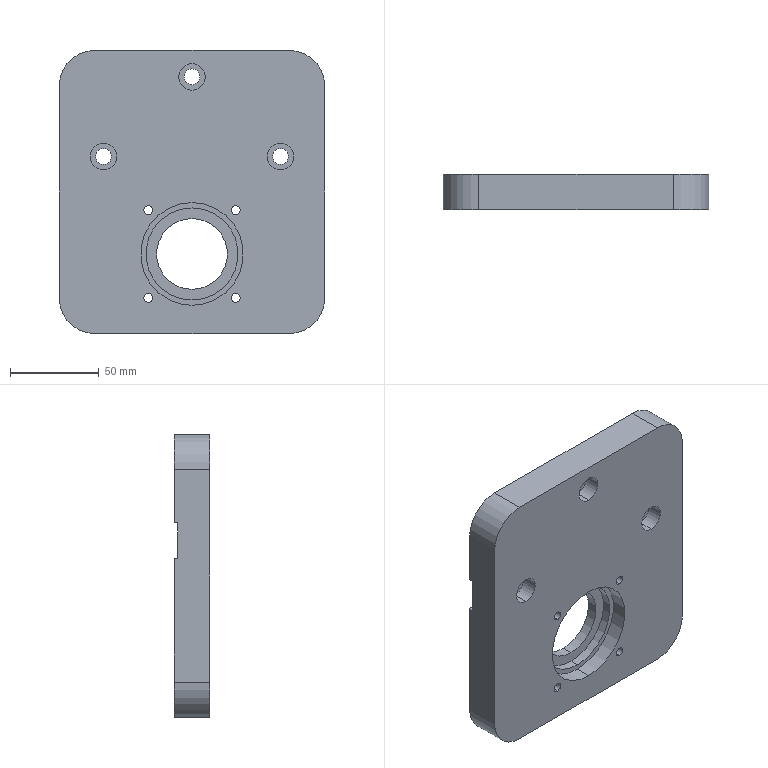Part | SolidWorks | features ICE 4, HoleWzd 2, Extrusion 1, Fillet 1 | 1 solid | 45 faces | box 150 x 20 x 160 mm | volume 417009 mm3 | cylinder 30 | plane 15 | commonest cylinder face diameters 5 x8 9 x6 15 x6 40 x6 52 x2 58 x2
STEP:
#1=CARTESIAN_POINT('',(125.,-11.,-52.5));
#2=VERTEX_POINT('',#1);
#3=CARTESIAN_POINT('',(125.,-11.,-67.5));
#4=VERTEX_POINT('',#3);
#5=CARTESIAN_POINT('',(125.,-11.,-60.));
#6=DIRECTION('',(0.,-1.,0.));
#7=DIRECTION('',(0.,0.,-1.));
#8=AXIS2_PLACEMENT_3D('',#5,#6,#7);
#9=CIRCLE('',#8,7.5);
#10=EDGE_CURVE('',#2,#4,#9,.T.);
#11=ORIENTED_EDGE('',*,*,#10,.F.);
#12=CARTESIAN_POINT('',(125.,-20.,-52.5));
#13=VERTEX_POINT('',#12);
#14=CARTESIAN_POINT('',(125.,-20.,-52.5));
#15=DIRECTION('',(0.,-1.,0.));
#16=VECTOR('',#15,1000.);
#17=LINE('',#14,#16);
#18=EDGE_CURVE('',#2,#13,#17,.T.);
#19=ORIENTED_EDGE('',*,*,#18,.T.);
#20=CARTESIAN_POINT('',(125.,-20.,-67.5));
#21=VERTEX_POINT('',#20);
#22=CARTESIAN_POINT('',(125.,-20.,-60.));
#23=DIRECTION('',(0.,-1.,0.));
#24=DIRECTION('',(0.,0.,-1.));
#25=AXIS2_PLACEMENT_3D('',#22,#23,#24);
#26=CIRCLE('',#25,7.5);
#27=EDGE_CURVE('',#13,#21,#26,.T.);
#28=ORIENTED_EDGE('',*,*,#27,.T.);
#29=CARTESIAN_POINT('',(125.,-20.,-67.5));
#30=DIRECTION('',(0.,-1.,0.));
#31=VECTOR('',#30,1000.);
#32=LINE('',#29,#31);
#33=EDGE_CURVE('',#4,#21,#32,.T.);
#34=ORIENTED_EDGE('',*,*,#33,.F.);
#35=EDGE_LOOP('',(#11,#19,#28,#34));
#36=FACE_OUTER_BOUND('',#35,.T.);
#37=CARTESIAN_POINT('',(125.,-20.,-60.));
#38=DIRECTION('',(0.,-1.,0.));
#39=DIRECTION('',(0.,0.,-1.));
#40=AXIS2_PLACEMENT_3D('',#37,#38,#39);
#41=CYLINDRICAL_SURFACE('',#40,7.5);
#42=ADVANCED_FACE('',(#36),#41,.F.);
#43=CARTESIAN_POINT('',(125.,-2.,-64.5));
#44=VERTEX_POINT('',#43);
#45=CARTESIAN_POINT('',(125.,-2.,-55.5));
#46=VERTEX_POINT('',#45);
#47=CARTESIAN_POINT('',(125.,-2.,-60.));
#48=DIRECTION('',(0.,1.,0.));
#49=DIRECTION('',(0.,0.,1.));
#50=AXIS2_PLACEMENT_3D('',#47,#48,#49);
#51=CIRCLE('',#50,4.5);
#52=EDGE_CURVE('',#44,#46,#51,.T.);
#53=ORIENTED_EDGE('',*,*,#52,.T.);
#54=CARTESIAN_POINT('',(125.,-11.,-55.5));
#55=VERTEX_POINT('',#54);
#56=CARTESIAN_POINT('',(125.,-20.,-55.5));
#57=DIRECTION('',(0.,-1.,0.));
#58=VECTOR('',#57,1000.);
#59=LINE('',#56,#58);
#60=EDGE_CURVE('',#46,#55,#59,.T.);
#61=ORIENTED_EDGE('',*,*,#60,.T.);
#62=CARTESIAN_POINT('',(125.,-11.,-64.5));
#63=VERTEX_POINT('',#62);
#64=CARTESIAN_POINT('',(125.,-11.,-60.));
#65=DIRECTION('',(0.,-1.,0.));
#66=DIRECTION('',(0.,0.,-1.));
#67=AXIS2_PLACEMENT_3D('',#64,#65,#66);
#68=CIRCLE('',#67,4.5);
#69=EDGE_CURVE('',#55,#63,#68,.T.);
#70=ORIENTED_EDGE('',*,*,#69,.T.);
#71=CARTESIAN_POINT('',(125.,-20.,-64.5));
#72=DIRECTION('',(0.,-1.,0.));
#73=VECTOR('',#72,1000.);
#74=LINE('',#71,#73);
#75=EDGE_CURVE('',#44,#63,#74,.T.);
#76=ORIENTED_EDGE('',*,*,#75,.F.);
#77=EDGE_LOOP('',(#53,#61,#70,#76));
#78=FACE_OUTER_BOUND('',#77,.T.);
#79=CARTESIAN_POINT('',(125.,-20.,-60.));
#80=DIRECTION('',(0.,-1.,0.));
#81=DIRECTION('',(0.,0.,-1.));
#82=AXIS2_PLACEMENT_3D('',#79,#80,#81);
#83=CYLINDRICAL_SURFACE('',#82,4.5);
#84=ADVANCED_FACE('',(#78),#83,.F.);
#85=CARTESIAN_POINT('',(25.,-11.,-52.5));
#86=VERTEX_POINT('',#85);
#87=CARTESIAN_POINT('',(25.,-11.,-67.5));
#88=VERTEX_POINT('',#87);
#89=CARTESIAN_POINT('',(25.,-11.,-60.));
#90=DIRECTION('',(0.,-1.,0.));
#91=DIRECTION('',(0.,0.,-1.));
#92=AXIS2_PLACEMENT_3D('',#89,#90,#91);
#93=CIRCLE('',#92,7.5);
#94=EDGE_CURVE('',#86,#88,#93,.T.);
#95=ORIENTED_EDGE('',*,*,#94,.F.);
#96=CARTESIAN_POINT('',(25.,-20.,-52.5));
#97=VERTEX_POINT('',#96);
#98=CARTESIAN_POINT('',(25.,-20.,-52.5));
#99=DIRECTION('',(0.,-1.,0.));
#100=VECTOR('',#99,1000.);
#101=LINE('',#98,#100);
#102=EDGE_CURVE('',#86,#97,#101,.T.);
#103=ORIENTED_EDGE('',*,*,#102,.T.);
#104=CARTESIAN_POINT('',(25.,-20.,-67.5));
#105=VERTEX_POINT('',#104);
#106=CARTESIAN_POINT('',(25.,-20.,-60.));
#107=DIRECTION('',(0.,-1.,0.));
#108=DIRECTION('',(0.,0.,-1.));
#109=AXIS2_PLACEMENT_3D('',#106,#107,#108);
#110=CIRCLE('',#109,7.5);
#111=EDGE_CURVE('',#97,#105,#110,.T.);
#112=ORIENTED_EDGE('',*,*,#111,.T.);
#113=CARTESIAN_POINT('',(25.,-20.,-67.5));
#114=DIRECTION('',(0.,-1.,0.));
#115=VECTOR('',#114,1000.);
#116=LINE('',#113,#115);
#117=EDGE_CURVE('',#88,#105,#116,.T.);
#118=ORIENTED_EDGE('',*,*,#117,.F.);
#119=EDGE_LOOP('',(#95,#103,#112,#118));
#120=FACE_OUTER_BOUND('',#119,.T.);
#121=CARTESIAN_POINT('',(25.,-20.,-60.));
#122=DIRECTION('',(0.,-1.,0.));
#123=DIRECTION('',(0.,0.,-1.));
#124=AXIS2_PLACEMENT_3D('',#121,#122,#123);
#125=CYLINDRICAL_SURFACE('',#124,7.5);
#126=ADVANCED_FACE('',(#120),#125,.F.);
#127=CARTESIAN_POINT('',(25.,-2.,-64.5));
#128=VERTEX_POINT('',#127);
#129=CARTESIAN_POINT('',(25.,-2.,-55.5));
#130=VERTEX_POINT('',#129);
#131=CARTESIAN_POINT('',(25.,-2.,-60.));
#132=DIRECTION('',(0.,1.,0.));
#133=DIRECTION('',(0.,0.,1.));
#134=AXIS2_PLACEMENT_3D('',#131,#132,#133);
#135=CIRCLE('',#134,4.5);
#136=EDGE_CURVE('',#128,#130,#135,.T.);
#137=ORIENTED_EDGE('',*,*,#136,.T.);
#138=CARTESIAN_POINT('',(25.,-11.,-55.5));
#139=VERTEX_POINT('',#138);
#140=CARTESIAN_POINT('',(25.,-20.,-55.5));
#141=DIRECTION('',(0.,-1.,0.));
#142=VECTOR('',#141,1000.);
#143=LINE('',#140,#142);
#144=EDGE_CURVE('',#130,#139,#143,.T.);
#145=ORIENTED_EDGE('',*,*,#144,.T.);
#146=CARTESIAN_POINT('',(25.,-11.,-64.5));
#147=VERTEX_POINT('',#146);
#148=CARTESIAN_POINT('',(25.,-11.,-60.));
#149=DIRECTION('',(0.,-1.,0.));
#150=DIRECTION('',(0.,0.,-1.));
#151=AXIS2_PLACEMENT_3D('',#148,#149,#150);
#152=CIRCLE('',#151,4.5);
#153=EDGE_CURVE('',#139,#147,#152,.T.);
#154=ORIENTED_EDGE('',*,*,#153,.T.);
#155=CARTESIAN_POINT('',(25.,-20.,-64.5));
#156=DIRECTION('',(0.,-1.,0.));
#157=VECTOR('',#156,1000.);
#158=LINE('',#155,#157);
#159=EDGE_CURVE('',#128,#147,#158,.T.);
#160=ORIENTED_EDGE('',*,*,#159,.F.);
#161=EDGE_LOOP('',(#137,#145,#154,#160));
#162=FACE_OUTER_BOUND('',#161,.T.);
#163=CARTESIAN_POINT('',(25.,-20.,-60.));
#164=DIRECTION('',(0.,-1.,0.));
#165=DIRECTION('',(0.,0.,-1.));
#166=AXIS2_PLACEMENT_3D('',#163,#164,#165);
#167=CYLINDRICAL_SURFACE('',#166,4.5);
#168=ADVANCED_FACE('',(#162),#167,.F.);
#169=CARTESIAN_POINT('',(75.,-11.,-7.5));
#170=VERTEX_POINT('',#169);
#171=CARTESIAN_POINT('',(75.,-11.,-22.5));
#172=VERTEX_POINT('',#171);
#173=CARTESIAN_POINT('',(75.,-11.,-15.));
#174=DIRECTION('',(0.,-1.,0.));
#175=DIRECTION('',(0.,0.,-1.));
#176=AXIS2_PLACEMENT_3D('',#173,#174,#175);
#177=CIRCLE('',#176,7.5);
#178=EDGE_CURVE('',#170,#172,#177,.T.);
#179=ORIENTED_EDGE('',*,*,#178,.F.);
#180=CARTESIAN_POINT('',(75.,-20.,-7.5));
#181=VERTEX_POINT('',#180);
#182=CARTESIAN_POINT('',(75.,-20.,-7.5));
#183=DIRECTION('',(0.,-1.,0.));
#184=VECTOR('',#183,1000.);
#185=LINE('',#182,#184);
#186=EDGE_CURVE('',#170,#181,#185,.T.);
#187=ORIENTED_EDGE('',*,*,#186,.T.);
#188=CARTESIAN_POINT('',(75.,-20.,-22.5));
#189=VERTEX_POINT('',#188);
#190=CARTESIAN_POINT('',(75.,-20.,-15.));
#191=DIRECTION('',(0.,-1.,0.));
#192=DIRECTION('',(0.,0.,-1.));
#193=AXIS2_PLACEMENT_3D('',#190,#191,#192);
#194=CIRCLE('',#193,7.5);
#195=EDGE_CURVE('',#181,#189,#194,.T.);
#196=ORIENTED_EDGE('',*,*,#195,.T.);
#197=CARTESIAN_POINT('',(75.,-20.,-22.5));
#198=DIRECTION('',(0.,-1.,0.));
#199=VECTOR('',#198,1000.);
#200=LINE('',#197,#199);
#201=EDGE_CURVE('',#172,#189,#200,.T.);
#202=ORIENTED_EDGE('',*,*,#201,.F.);
#203=EDGE_LOOP('',(#179,#187,#196,#202));
#204=FACE_OUTER_BOUND('',#203,.T.);
#205=CARTESIAN_POINT('',(75.,-20.,-15.));
#206=DIRECTION('',(0.,-1.,0.));
#207=DIRECTION('',(0.,0.,-1.));
#208=AXIS2_PLACEMENT_3D('',#205,#206,#207);
#209=CYLINDRICAL_SURFACE('',#208,7.5);
#210=ADVANCED_FACE('',(#204),#209,.F.);
#211=CARTESIAN_POINT('',(75.,0.,-10.5));
#212=VERTEX_POINT('',#211);
#213=CARTESIAN_POINT('',(75.,0.,-19.5));
#214=VERTEX_POINT('',#213);
#215=CARTESIAN_POINT('',(75.,0.,-15.));
#216=DIRECTION('',(0.,-1.,0.));
#217=DIRECTION('',(0.,0.,-1.));
#218=AXIS2_PLACEMENT_3D('',#215,#216,#217);
#219=CIRCLE('',#218,4.5);
#220=EDGE_CURVE('',#212,#214,#219,.T.);
#221=ORIENTED_EDGE('',*,*,#220,.F.);
#222=CARTESIAN_POINT('',(75.,-11.,-10.5));
#223=VERTEX_POINT('',#222);
#224=CARTESIAN_POINT('',(75.,-20.,-10.5));
#225=DIRECTION('',(0.,-1.,0.));
#226=VECTOR('',#225,1000.);
#227=LINE('',#224,#226);
#228=EDGE_CURVE('',#212,#223,#227,.T.);
#229=ORIENTED_EDGE('',*,*,#228,.T.);
#230=CARTESIAN_POINT('',(75.,-11.,-19.5));
#231=VERTEX_POINT('',#230);
#232=CARTESIAN_POINT('',(75.,-11.,-15.));
#233=DIRECTION('',(0.,-1.,0.));
#234=DIRECTION('',(0.,0.,-1.));
#235=AXIS2_PLACEMENT_3D('',#232,#233,#234);
#236=CIRCLE('',#235,4.5);
#237=EDGE_CURVE('',#223,#231,#236,.T.);
#238=ORIENTED_EDGE('',*,*,#237,.T.);
#239=CARTESIAN_POINT('',(75.,-20.,-19.5));
#240=DIRECTION('',(0.,-1.,0.));
#241=VECTOR('',#240,1000.);
#242=LINE('',#239,#241);
#243=EDGE_CURVE('',#214,#231,#242,.T.);
#244=ORIENTED_EDGE('',*,*,#243,.F.);
#245=EDGE_LOOP('',(#221,#229,#238,#244));
#246=FACE_OUTER_BOUND('',#245,.T.);
#247=CARTESIAN_POINT('',(75.,-20.,-15.));
#248=DIRECTION('',(0.,-1.,0.));
#249=DIRECTION('',(0.,0.,-1.));
#250=AXIS2_PLACEMENT_3D('',#247,#248,#249);
#251=CYLINDRICAL_SURFACE('',#250,4.5);
#252=ADVANCED_FACE('',(#246),#251,.F.);
#253=CARTESIAN_POINT('',(75.,-11.,-86.));
#254=VERTEX_POINT('',#253);
#255=CARTESIAN_POINT('',(75.,-11.,-144.));
#256=VERTEX_POINT('',#255);
#257=CARTESIAN_POINT('',(75.,-11.,-115.));
#258=DIRECTION('',(0.,-1.,0.));
#259=DIRECTION('',(0.,0.,-1.));
#260=AXIS2_PLACEMENT_3D('',#257,#258,#259);
#261=CIRCLE('',#260,29.);
#262=EDGE_CURVE('',#254,#256,#261,.T.);
#263=ORIENTED_EDGE('',*,*,#262,.F.);
#264=CARTESIAN_POINT('',(75.,-20.,-86.));
#265=VERTEX_POINT('',#264);
#266=CARTESIAN_POINT('',(75.,-11.,-86.));
#267=DIRECTION('',(0.,-1.,0.));
#268=VECTOR('',#267,1000.);
#269=LINE('',#266,#268);
#270=EDGE_CURVE('',#254,#265,#269,.T.);
#271=ORIENTED_EDGE('',*,*,#270,.T.);
#272=CARTESIAN_POINT('',(75.,-20.,-144.));
#273=VERTEX_POINT('',#272);
#274=CARTESIAN_POINT('',(75.,-20.,-115.));
#275=DIRECTION('',(0.,-1.,0.));
#276=DIRECTION('',(0.,0.,-1.));
#277=AXIS2_PLACEMENT_3D('',#274,#275,#276);
#278=CIRCLE('',#277,29.);
#279=EDGE_CURVE('',#265,#273,#278,.T.);
#280=ORIENTED_EDGE('',*,*,#279,.T.);
#281=CARTESIAN_POINT('',(75.,-11.,-144.));
#282=DIRECTION('',(0.,-1.,0.));
#283=VECTOR('',#282,1000.);
#284=LINE('',#281,#283);
#285=EDGE_CURVE('',#256,#273,#284,.T.);
#286=ORIENTED_EDGE('',*,*,#285,.F.);
#287=EDGE_LOOP('',(#263,#271,#280,#286));
#288=FACE_OUTER_BOUND('',#287,.T.);
#289=CARTESIAN_POINT('',(75.,-11.,-115.));
#290=DIRECTION('',(0.,-1.,0.));
#291=DIRECTION('',(0.,0.,-1.));
#292=AXIS2_PLACEMENT_3D('',#289,#290,#291);
#293=CYLINDRICAL_SURFACE('',#292,29.);
#294=ADVANCED_FACE('',(#288),#293,.F.);
#295=CARTESIAN_POINT('',(99.749,0.,-137.249));
#296=VERTEX_POINT('',#295);
#297=CARTESIAN_POINT('',(99.749,0.,-142.249));
#298=VERTEX_POINT('',#297);
#299=CARTESIAN_POINT('',(99.749,0.,-139.749));
#300=DIRECTION('',(0.,-1.,0.));
#301=DIRECTION('',(0.,0.,-1.));
#302=AXIS2_PLACEMENT_3D('',#299,#300,#301);
#303=CIRCLE('',#302,2.5);
#304=EDGE_CURVE('',#296,#298,#303,.T.);
#305=ORIENTED_EDGE('',*,*,#304,.F.);
#306=CARTESIAN_POINT('',(99.749,-20.,-137.249));
#307=VERTEX_POINT('',#306);
#308=CARTESIAN_POINT('',(99.749,-20.,-137.249));
#309=DIRECTION('',(0.,-1.,0.));
#310=VECTOR('',#309,1000.);
#311=LINE('',#308,#310);
#312=EDGE_CURVE('',#296,#307,#311,.T.);
#313=ORIENTED_EDGE('',*,*,#312,.T.);
#314=CARTESIAN_POINT('',(99.749,-20.,-142.249));
#315=VERTEX_POINT('',#314);
#316=CARTESIAN_POINT('',(99.749,-20.,-139.749));
#317=DIRECTION('',(0.,-1.,0.));
#318=DIRECTION('',(0.,0.,-1.));
#319=AXIS2_PLACEMENT_3D('',#316,#317,#318);
#320=CIRCLE('',#319,2.5);
#321=EDGE_CURVE('',#307,#315,#320,.T.);
#322=ORIENTED_EDGE('',*,*,#321,.T.);
#323=CARTESIAN_POINT('',(99.749,-20.,-142.249));
#324=DIRECTION('',(0.,-1.,0.));
#325=VECTOR('',#324,1000.);
#326=LINE('',#323,#325);
#327=EDGE_CURVE('',#298,#315,#326,.T.);
#328=ORIENTED_EDGE('',*,*,#327,.F.);
#329=EDGE_LOOP('',(#305,#313,#322,#328));
#330=FACE_OUTER_BOUND('',#329,.T.);
#331=CARTESIAN_POINT('',(99.749,-20.,-139.749));
#332=DIRECTION('',(0.,-1.,0.));
#333=DIRECTION('',(0.,0.,-1.));
#334=AXIS2_PLACEMENT_3D('',#331,#332,#333);
#335=CYLINDRICAL_SURFACE('',#334,2.5);
#336=ADVANCED_FACE('',(#330),#335,.F.);
#337=CARTESIAN_POINT('',(50.251,0.,-137.249));
#338=VERTEX_POINT('',#337);
#339=CARTESIAN_POINT('',(50.251,0.,-142.249));
#340=VERTEX_POINT('',#339);
#341=CARTESIAN_POINT('',(50.251,0.,-139.749));
#342=DIRECTION('',(0.,-1.,0.));
#343=DIRECTION('',(0.,0.,-1.));
#344=AXIS2_PLACEMENT_3D('',#341,#342,#343);
#345=CIRCLE('',#344,2.5);
#346=EDGE_CURVE('',#338,#340,#345,.T.);
#347=ORIENTED_EDGE('',*,*,#346,.F.);
#348=CARTESIAN_POINT('',(50.251,-20.,-137.249));
#349=VERTEX_POINT('',#348);
#350=CARTESIAN_POINT('',(50.251,-20.,-137.249));
#351=DIRECTION('',(0.,-1.,0.));
#352=VECTOR('',#351,1000.);
#353=LINE('',#350,#352);
#354=EDGE_CURVE('',#338,#349,#353,.T.);
#355=ORIENTED_EDGE('',*,*,#354,.T.);
#356=CARTESIAN_POINT('',(50.251,-20.,-142.249));
#357=VERTEX_POINT('',#356);
#358=CARTESIAN_POINT('',(50.251,-20.,-139.749));
#359=DIRECTION('',(0.,-1.,0.));
#360=DIRECTION('',(0.,0.,-1.));
#361=AXIS2_PLACEMENT_3D('',#358,#359,#360);
#362=CIRCLE('',#361,2.5);
#363=EDGE_CURVE('',#349,#357,#362,.T.);
#364=ORIENTED_EDGE('',*,*,#363,.T.);
#365=CARTESIAN_POINT('',(50.251,-20.,-142.249));
#366=DIRECTION('',(0.,-1.,0.));
#367=VECTOR('',#366,1000.);
#368=LINE('',#365,#367);
#369=EDGE_CURVE('',#340,#357,#368,.T.);
#370=ORIENTED_EDGE('',*,*,#369,.F.);
#371=EDGE_LOOP('',(#347,#355,#364,#370));
#372=FACE_OUTER_BOUND('',#371,.T.);
#373=CARTESIAN_POINT('',(50.251,-20.,-139.749));
#374=DIRECTION('',(0.,-1.,0.));
#375=DIRECTION('',(0.,0.,-1.));
#376=AXIS2_PLACEMENT_3D('',#373,#374,#375);
#377=CYLINDRICAL_SURFACE('',#376,2.5);
#378=ADVANCED_FACE('',(#372),#377,.F.);
#379=CARTESIAN_POINT('',(50.251,0.,-87.751));
#380=VERTEX_POINT('',#379);
#381=CARTESIAN_POINT('',(50.251,0.,-92.751));
#382=VERTEX_POINT('',#381);
#383=CARTESIAN_POINT('',(50.251,0.,-90.251));
#384=DIRECTION('',(0.,-1.,0.));
#385=DIRECTION('',(0.,0.,-1.));
#386=AXIS2_PLACEMENT_3D('',#383,#384,#385);
#387=CIRCLE('',#386,2.5);
#388=EDGE_CURVE('',#380,#382,#387,.T.);
#389=ORIENTED_EDGE('',*,*,#388,.F.);
#390=CARTESIAN_POINT('',(50.251,-20.,-87.751));
#391=VERTEX_POINT('',#390);
#392=CARTESIAN_POINT('',(50.251,-20.,-87.751));
#393=DIRECTION('',(0.,-1.,0.));
#394=VECTOR('',#393,1000.);
#395=LINE('',#392,#394);
#396=EDGE_CURVE('',#380,#391,#395,.T.);
#397=ORIENTED_EDGE('',*,*,#396,.T.);
#398=CARTESIAN_POINT('',(50.251,-20.,-92.751));
#399=VERTEX_POINT('',#398);
#400=CARTESIAN_POINT('',(50.251,-20.,-90.251));
#401=DIRECTION('',(0.,-1.,0.));
#402=DIRECTION('',(0.,0.,-1.));
#403=AXIS2_PLACEMENT_3D('',#400,#401,#402);
#404=CIRCLE('',#403,2.5);
#405=EDGE_CURVE('',#391,#399,#404,.T.);
#406=ORIENTED_EDGE('',*,*,#405,.T.);
#407=CARTESIAN_POINT('',(50.251,-20.,-92.751));
#408=DIRECTION('',(0.,-1.,0.));
#409=VECTOR('',#408,1000.);
#410=LINE('',#407,#409);
#411=EDGE_CURVE('',#382,#399,#410,.T.);
#412=ORIENTED_EDGE('',*,*,#411,.F.);
#413=EDGE_LOOP('',(#389,#397,#406,#412));
#414=FACE_OUTER_BOUND('',#413,.T.);
#415=CARTESIAN_POINT('',(50.251,-20.,-90.251));
#416=DIRECTION('',(0.,-1.,0.));
#417=DIRECTION('',(0.,0.,-1.));
#418=AXIS2_PLACEMENT_3D('',#415,#416,#417);
#419=CYLINDRICAL_SURFACE('',#418,2.5);
#420=ADVANCED_FACE('',(#414),#419,.F.);
#421=CARTESIAN_POINT('',(99.749,0.,-87.751));
#422=VERTEX_POINT('',#421);
#423=CARTESIAN_POINT('',(99.749,0.,-92.751));
#424=VERTEX_POINT('',#423);
#425=CARTESIAN_POINT('',(99.749,0.,-90.251));
#426=DIRECTION('',(0.,-1.,0.));
#427=DIRECTION('',(0.,0.,-1.));
#428=AXIS2_PLACEMENT_3D('',#425,#426,#427);
#429=CIRCLE('',#428,2.5);
#430=EDGE_CURVE('',#422,#424,#429,.T.);
#431=ORIENTED_EDGE('',*,*,#430,.F.);
#432=CARTESIAN_POINT('',(99.749,-20.,-87.751));
#433=VERTEX_POINT('',#432);
#434=CARTESIAN_POINT('',(99.749,-20.,-87.751));
#435=DIRECTION('',(0.,-1.,0.));
#436=VECTOR('',#435,1000.);
#437=LINE('',#434,#436);
#438=EDGE_CURVE('',#422,#433,#437,.T.);
#439=ORIENTED_EDGE('',*,*,#438,.T.);
#440=CARTESIAN_POINT('',(99.749,-20.,-92.751));
#441=VERTEX_POINT('',#440);
#442=CARTESIAN_POINT('',(99.749,-20.,-90.251));
#443=DIRECTION('',(0.,-1.,0.));
#444=DIRECTION('',(0.,0.,-1.));
#445=AXIS2_PLACEMENT_3D('',#442,#443,#444);
#446=CIRCLE('',#445,2.5);
#447=EDGE_CURVE('',#433,#441,#446,.T.);
#448=ORIENTED_EDGE('',*,*,#447,.T.);
#449=CARTESIAN_POINT('',(99.749,-20.,-92.751));
#450=DIRECTION('',(0.,-1.,0.));
#451=VECTOR('',#450,1000.);
#452=LINE('',#449,#451);
#453=EDGE_CURVE('',#424,#441,#452,.T.);
#454=ORIENTED_EDGE('',*,*,#453,.F.);
#455=EDGE_LOOP('',(#431,#439,#448,#454));
#456=FACE_OUTER_BOUND('',#455,.T.);
#457=CARTESIAN_POINT('',(99.749,-20.,-90.251));
#458=DIRECTION('',(0.,-1.,0.));
#459=DIRECTION('',(0.,0.,-1.));
#460=AXIS2_PLACEMENT_3D('',#457,#458,#459);
#461=CYLINDRICAL_SURFACE('',#460,2.5);
#462=ADVANCED_FACE('',(#456),#461,.F.);
#463=CARTESIAN_POINT('',(75.,0.,-95.));
#464=VERTEX_POINT('',#463);
#465=CARTESIAN_POINT('',(75.,0.,-135.));
#466=VERTEX_POINT('',#465);
#467=CARTESIAN_POINT('',(75.,0.,-115.));
#468=DIRECTION('',(0.,-1.,0.));
#469=DIRECTION('',(0.,0.,-1.));
#470=AXIS2_PLACEMENT_3D('',#467,#468,#469);
#471=CIRCLE('',#470,20.);
#472=EDGE_CURVE('',#464,#466,#471,.T.);
#473=ORIENTED_EDGE('',*,*,#472,.F.);
#474=CARTESIAN_POINT('',(75.,-6.,-95.));
#475=VERTEX_POINT('',#474);
#476=CARTESIAN_POINT('',(75.,8.,-95.));
#477=DIRECTION('',(0.,-1.,0.));
#478=VECTOR('',#477,1000.);
#479=LINE('',#476,#478);
#480=EDGE_CURVE('',#464,#475,#479,.T.);
#481=ORIENTED_EDGE('',*,*,#480,.T.);
#482=CARTESIAN_POINT('',(75.,-6.,-135.));
#483=VERTEX_POINT('',#482);
#484=CARTESIAN_POINT('',(75.,-6.,-115.));
#485=DIRECTION('',(0.,-1.,0.));
#486=DIRECTION('',(0.,0.,-1.));
#487=AXIS2_PLACEMENT_3D('',#484,#485,#486);
#488=CIRCLE('',#487,20.);
#489=EDGE_CURVE('',#475,#483,#488,.T.);
#490=ORIENTED_EDGE('',*,*,#489,.T.);
#491=CARTESIAN_POINT('',(75.,8.,-135.));
#492=DIRECTION('',(0.,-1.,0.));
#493=VECTOR('',#492,1000.);
#494=LINE('',#491,#493);
#495=EDGE_CURVE('',#466,#483,#494,.T.);
#496=ORIENTED_EDGE('',*,*,#495,.F.);
#497=EDGE_LOOP('',(#473,#481,#490,#496));
#498=FACE_OUTER_BOUND('',#497,.T.);
#499=CARTESIAN_POINT('',(75.,8.,-115.));
#500=DIRECTION('',(0.,-1.,0.));
#501=DIRECTION('',(0.,0.,-1.));
#502=AXIS2_PLACEMENT_3D('',#499,#500,#501);
#503=CYLINDRICAL_SURFACE('',#502,20.);
#504=ADVANCED_FACE('',(#498),#503,.F.);
#505=CARTESIAN_POINT('',(75.,-6.,-89.));
#506=VERTEX_POINT('',#505);
#507=CARTESIAN_POINT('',(75.,-6.,-141.));
#508=VERTEX_POINT('',#507);
#509=CARTESIAN_POINT('',(75.,-6.,-115.));
#510=DIRECTION('',(0.,-1.,0.));
#511=DIRECTION('',(0.,0.,-1.));
#512=AXIS2_PLACEMENT_3D('',#509,#510,#511);
#513=CIRCLE('',#512,26.);
#514=EDGE_CURVE('',#506,#508,#513,.T.);
#515=ORIENTED_EDGE('',*,*,#514,.F.);
#516=CARTESIAN_POINT('',(75.,-11.,-89.));
#517=VERTEX_POINT('',#516);
#518=CARTESIAN_POINT('',(75.,-6.,-89.));
#519=DIRECTION('',(0.,-1.,0.));
#520=VECTOR('',#519,1000.);
#521=LINE('',#518,#520);
#522=EDGE_CURVE('',#506,#517,#521,.T.);
#523=ORIENTED_EDGE('',*,*,#522,.T.);
#524=CARTESIAN_POINT('',(75.,-11.,-141.));
#525=VERTEX_POINT('',#524);
#526=CARTESIAN_POINT('',(75.,-11.,-115.));
#527=DIRECTION('',(0.,1.,0.));
#528=DIRECTION('',(0.,0.,-1.));
#529=AXIS2_PLACEMENT_3D('',#526,#527,#528);
#530=CIRCLE('',#529,26.);
#531=EDGE_CURVE('',#525,#517,#530,.T.);
#532=ORIENTED_EDGE('',*,*,#531,.F.);
#533=CARTESIAN_POINT('',(75.,-6.,-141.));
#534=DIRECTION('',(0.,-1.,0.));
#535=VECTOR('',#534,1000.);
#536=LINE('',#533,#535);
#537=EDGE_CURVE('',#508,#525,#536,.T.);
#538=ORIENTED_EDGE('',*,*,#537,.F.);
#539=EDGE_LOOP('',(#515,#523,#532,#538));
#540=FACE_OUTER_BOUND('',#539,.T.);
#541=CARTESIAN_POINT('',(75.,-6.,-115.));
#542=DIRECTION('',(0.,-1.,0.));
#543=DIRECTION('',(0.,0.,-1.));
#544=AXIS2_PLACEMENT_3D('',#541,#542,#543);
#545=CYLINDRICAL_SURFACE('',#544,26.);
#546=ADVANCED_FACE('',(#540),#545,.F.);
#547=CARTESIAN_POINT('',(75.,0.,-115.));
#548=DIRECTION('',(0.,-1.,0.));
#549=DIRECTION('',(0.,0.,-1.));
#550=AXIS2_PLACEMENT_3D('',#547,#548,#549);
#551=CIRCLE('',#550,20.);
#552=EDGE_CURVE('',#466,#464,#551,.T.);
#553=ORIENTED_EDGE('',*,*,#552,.T.);
#554=ORIENTED_EDGE('',*,*,#472,.T.);
#555=EDGE_LOOP('',(#553,#554));
#556=FACE_BOUND('',#555,.T.);
#557=CARTESIAN_POINT('',(99.749,0.,-90.251));
#558=DIRECTION('',(0.,-1.,0.));
#559=DIRECTION('',(0.,0.,-1.));
#560=AXIS2_PLACEMENT_3D('',#557,#558,#559);
#561=CIRCLE('',#560,2.5);
#562=EDGE_CURVE('',#424,#422,#561,.T.);
#563=ORIENTED_EDGE('',*,*,#562,.T.);
#564=ORIENTED_EDGE('',*,*,#430,.T.);
#565=EDGE_LOOP('',(#563,#564));
#566=FACE_BOUND('',#565,.T.);
#567=CARTESIAN_POINT('',(50.251,0.,-90.251));
#568=DIRECTION('',(0.,-1.,0.));
#569=DIRECTION('',(0.,0.,-1.));
#570=AXIS2_PLACEMENT_3D('',#567,#568,#569);
#571=CIRCLE('',#570,2.5);
#572=EDGE_CURVE('',#382,#380,#571,.T.);
#573=ORIENTED_EDGE('',*,*,#572,.T.);
#574=ORIENTED_EDGE('',*,*,#388,.T.);
#575=EDGE_LOOP('',(#573,#574));
#576=FACE_BOUND('',#575,.T.);
#577=CARTESIAN_POINT('',(50.251,0.,-139.749));
#578=DIRECTION('',(0.,-1.,0.));
#579=DIRECTION('',(0.,0.,-1.));
#580=AXIS2_PLACEMENT_3D('',#577,#578,#579);
#581=CIRCLE('',#580,2.5);
#582=EDGE_CURVE('',#340,#338,#581,.T.);
#583=ORIENTED_EDGE('',*,*,#582,.T.);
#584=ORIENTED_EDGE('',*,*,#346,.T.);
#585=EDGE_LOOP('',(#583,#584));
#586=FACE_BOUND('',#585,.T.);
#587=CARTESIAN_POINT('',(99.749,0.,-139.749));
#588=DIRECTION('',(0.,-1.,0.));
#589=DIRECTION('',(0.,0.,-1.));
#590=AXIS2_PLACEMENT_3D('',#587,#588,#589);
#591=CIRCLE('',#590,2.5);
#592=EDGE_CURVE('',#298,#296,#591,.T.);
#593=ORIENTED_EDGE('',*,*,#592,.T.);
#594=ORIENTED_EDGE('',*,*,#304,.T.);
#595=EDGE_LOOP('',(#593,#594));
#596=FACE_BOUND('',#595,.T.);
#597=CARTESIAN_POINT('',(0.,0.,-70.));
#598=VERTEX_POINT('',#597);
#599=CARTESIAN_POINT('',(0.,0.,-140.));
#600=VERTEX_POINT('',#599);
#601=CARTESIAN_POINT('',(0.,0.,0.));
#602=DIRECTION('',(0.,0.,-1.));
#603=VECTOR('',#602,1000.);
#604=LINE('',#601,#603);
#605=EDGE_CURVE('',#598,#600,#604,.T.);
#606=ORIENTED_EDGE('',*,*,#605,.F.);
#607=CARTESIAN_POINT('',(150.,0.,-70.));
#608=VERTEX_POINT('',#607);
#609=CARTESIAN_POINT('',(0.,0.,-70.));
#610=DIRECTION('',(-1.,0.,0.));
#611=VECTOR('',#610,1000.);
#612=LINE('',#609,#611);
#613=EDGE_CURVE('',#608,#598,#612,.T.);
#614=ORIENTED_EDGE('',*,*,#613,.F.);
#615=CARTESIAN_POINT('',(150.,0.,-140.));
#616=VERTEX_POINT('',#615);
#617=CARTESIAN_POINT('',(150.,0.,0.));
#618=DIRECTION('',(0.,0.,1.));
#619=VECTOR('',#618,1000.);
#620=LINE('',#617,#619);
#621=EDGE_CURVE('',#616,#608,#620,.T.);
#622=ORIENTED_EDGE('',*,*,#621,.F.);
#623=CARTESIAN_POINT('',(130.,0.,-160.));
#624=VERTEX_POINT('',#623);
#625=CARTESIAN_POINT('',(130.,0.,-140.));
#626=DIRECTION('',(0.,1.,0.));
#627=DIRECTION('',(0.,0.,-1.));
#628=AXIS2_PLACEMENT_3D('',#625,#626,#627);
#629=CIRCLE('',#628,20.);
#630=EDGE_CURVE('',#616,#624,#629,.T.);
#631=ORIENTED_EDGE('',*,*,#630,.T.);
#632=CARTESIAN_POINT('',(20.,0.,-160.));
#633=VERTEX_POINT('',#632);
#634=CARTESIAN_POINT('',(0.,0.,-160.));
#635=DIRECTION('',(1.,0.,0.));
#636=VECTOR('',#635,1000.);
#637=LINE('',#634,#636);
#638=EDGE_CURVE('',#633,#624,#637,.T.);
#639=ORIENTED_EDGE('',*,*,#638,.F.);
#640=CARTESIAN_POINT('',(20.,0.,-140.));
#641=DIRECTION('',(0.,1.,0.));
#642=DIRECTION('',(0.,0.,-1.));
#643=AXIS2_PLACEMENT_3D('',#640,#641,#642);
#644=CIRCLE('',#643,20.);
#645=EDGE_CURVE('',#633,#600,#644,.T.);
#646=ORIENTED_EDGE('',*,*,#645,.T.);
#647=EDGE_LOOP('',(#606,#614,#622,#631,#639,#646));
#648=FACE_OUTER_BOUND('',#647,.T.);
#649=CARTESIAN_POINT('',(0.,0.,0.));
#650=DIRECTION('',(0.,-1.,0.));
#651=DIRECTION('',(0.,0.,-1.));
#652=AXIS2_PLACEMENT_3D('',#649,#650,#651);
#653=PLANE('',#652);
#654=ADVANCED_FACE('',(#556,#566,#576,#586,#596,#648),#653,.F.);
#655=ORIENTED_EDGE('',*,*,#522,.F.);
#656=CARTESIAN_POINT('',(75.,-6.,-115.));
#657=DIRECTION('',(0.,-1.,0.));
#658=DIRECTION('',(0.,0.,-1.));
#659=AXIS2_PLACEMENT_3D('',#656,#657,#658);
#660=CIRCLE('',#659,26.);
#661=EDGE_CURVE('',#508,#506,#660,.T.);
#662=ORIENTED_EDGE('',*,*,#661,.F.);
#663=ORIENTED_EDGE('',*,*,#537,.T.);
#664=CARTESIAN_POINT('',(75.,-11.,-115.));
#665=DIRECTION('',(0.,1.,0.));
#666=DIRECTION('',(0.,0.,-1.));
#667=AXIS2_PLACEMENT_3D('',#664,#665,#666);
#668=CIRCLE('',#667,26.);
#669=EDGE_CURVE('',#517,#525,#668,.T.);
#670=ORIENTED_EDGE('',*,*,#669,.F.);
#671=EDGE_LOOP('',(#655,#662,#663,#670));
#672=FACE_OUTER_BOUND('',#671,.T.);
#673=CARTESIAN_POINT('',(75.,-6.,-115.));
#674=DIRECTION('',(0.,-1.,0.));
#675=DIRECTION('',(0.,0.,-1.));
#676=AXIS2_PLACEMENT_3D('',#673,#674,#675);
#677=CYLINDRICAL_SURFACE('',#676,26.);
#678=ADVANCED_FACE('',(#672),#677,.F.);
#679=CARTESIAN_POINT('',(0.,-2.,-70.));
#680=VERTEX_POINT('',#679);
#681=CARTESIAN_POINT('',(0.,-2.,-50.));
#682=VERTEX_POINT('',#681);
#683=CARTESIAN_POINT('',(0.,-2.,-70.));
#684=DIRECTION('',(0.,0.,1.));
#685=VECTOR('',#684,1000.);
#686=LINE('',#683,#685);
#687=EDGE_CURVE('',#680,#682,#686,.T.);
#688=ORIENTED_EDGE('',*,*,#687,.F.);
#689=CARTESIAN_POINT('',(0.,-2.,-70.));
#690=DIRECTION('',(0.,1.,0.));
#691=VECTOR('',#690,1000.);
#692=LINE('',#689,#691);
#693=EDGE_CURVE('',#680,#598,#692,.T.);
#694=ORIENTED_EDGE('',*,*,#693,.T.);
#695=ORIENTED_EDGE('',*,*,#605,.T.);
#696=CARTESIAN_POINT('',(0.,-20.,-140.));
#697=VERTEX_POINT('',#696);
#698=CARTESIAN_POINT('',(0.,-20.,-140.));
#699=DIRECTION('',(0.,-1.,0.));
#700=VECTOR('',#699,1000.);
#701=LINE('',#698,#700);
#702=EDGE_CURVE('',#600,#697,#701,.T.);
#703=ORIENTED_EDGE('',*,*,#702,.T.);
#704=CARTESIAN_POINT('',(0.,-20.,-20.));
#705=VERTEX_POINT('',#704);
#706=CARTESIAN_POINT('',(0.,-20.,0.));
#707=DIRECTION('',(0.,0.,-1.));
#708=VECTOR('',#707,1000.);
#709=LINE('',#706,#708);
#710=EDGE_CURVE('',#705,#697,#709,.T.);
#711=ORIENTED_EDGE('',*,*,#710,.F.);
#712=CARTESIAN_POINT('',(0.,0.,-20.));
#713=VERTEX_POINT('',#712);
#714=CARTESIAN_POINT('',(0.,-20.,-20.));
#715=DIRECTION('',(0.,1.,0.));
#716=VECTOR('',#715,1000.);
#717=LINE('',#714,#716);
#718=EDGE_CURVE('',#705,#713,#717,.T.);
#719=ORIENTED_EDGE('',*,*,#718,.T.);
#720=CARTESIAN_POINT('',(0.,0.,-50.));
#721=VERTEX_POINT('',#720);
#722=CARTESIAN_POINT('',(0.,0.,0.));
#723=DIRECTION('',(0.,0.,-1.));
#724=VECTOR('',#723,1000.);
#725=LINE('',#722,#724);
#726=EDGE_CURVE('',#713,#721,#725,.T.);
#727=ORIENTED_EDGE('',*,*,#726,.T.);
#728=CARTESIAN_POINT('',(0.,-2.,-50.));
#729=DIRECTION('',(0.,1.,0.));
#730=VECTOR('',#729,1000.);
#731=LINE('',#728,#730);
#732=EDGE_CURVE('',#682,#721,#731,.T.);
#733=ORIENTED_EDGE('',*,*,#732,.F.);
#734=EDGE_LOOP('',(#688,#694,#695,#703,#711,#719,#727,#733));
#735=FACE_OUTER_BOUND('',#734,.T.);
#736=CARTESIAN_POINT('',(0.,-20.,0.));
#737=DIRECTION('',(1.,0.,0.));
#738=DIRECTION('',(0.,0.,-1.));
#739=AXIS2_PLACEMENT_3D('',#736,#737,#738);
#740=PLANE('',#739);
#741=ADVANCED_FACE('',(#735),#740,.F.);
#742=ORIENTED_EDGE('',*,*,#638,.T.);
#743=CARTESIAN_POINT('',(130.,-20.,-160.));
#744=VERTEX_POINT('',#743);
#745=CARTESIAN_POINT('',(130.,-20.,-160.));
#746=DIRECTION('',(0.,-1.,0.));
#747=VECTOR('',#746,1000.);
#748=LINE('',#745,#747);
#749=EDGE_CURVE('',#624,#744,#748,.T.);
#750=ORIENTED_EDGE('',*,*,#749,.T.);
#751=CARTESIAN_POINT('',(20.,-20.,-160.));
#752=VERTEX_POINT('',#751);
#753=CARTESIAN_POINT('',(0.,-20.,-160.));
#754=DIRECTION('',(1.,0.,0.));
#755=VECTOR('',#754,1000.);
#756=LINE('',#753,#755);
#757=EDGE_CURVE('',#752,#744,#756,.T.);
#758=ORIENTED_EDGE('',*,*,#757,.F.);
#759=CARTESIAN_POINT('',(20.,-20.,-160.));
#760=DIRECTION('',(0.,1.,0.));
#761=VECTOR('',#760,1000.);
#762=LINE('',#759,#761);
#763=EDGE_CURVE('',#752,#633,#762,.T.);
#764=ORIENTED_EDGE('',*,*,#763,.T.);
#765=EDGE_LOOP('',(#742,#750,#758,#764));
#766=FACE_OUTER_BOUND('',#765,.T.);
#767=CARTESIAN_POINT('',(0.,-20.,-160.));
#768=DIRECTION('',(0.,0.,1.));
#769=DIRECTION('',(1.,0.,0.));
#770=AXIS2_PLACEMENT_3D('',#767,#768,#769);
#771=PLANE('',#770);
#772=ADVANCED_FACE('',(#766),#771,.F.);
#773=ORIENTED_EDGE('',*,*,#621,.T.);
#774=CARTESIAN_POINT('',(150.,-2.,-70.));
#775=VERTEX_POINT('',#774);
#776=CARTESIAN_POINT('',(150.,-2.,-70.));
#777=DIRECTION('',(0.,1.,0.));
#778=VECTOR('',#777,1000.);
#779=LINE('',#776,#778);
#780=EDGE_CURVE('',#775,#608,#779,.T.);
#781=ORIENTED_EDGE('',*,*,#780,.F.);
#782=CARTESIAN_POINT('',(150.,-2.,-50.));
#783=VERTEX_POINT('',#782);
#784=CARTESIAN_POINT('',(150.,-2.,-70.));
#785=DIRECTION('',(0.,0.,-1.));
#786=VECTOR('',#785,1000.);
#787=LINE('',#784,#786);
#788=EDGE_CURVE('',#783,#775,#787,.T.);
#789=ORIENTED_EDGE('',*,*,#788,.F.);
#790=CARTESIAN_POINT('',(150.,0.,-50.));
#791=VERTEX_POINT('',#790);
#792=CARTESIAN_POINT('',(150.,-2.,-50.));
#793=DIRECTION('',(0.,1.,0.));
#794=VECTOR('',#793,1000.);
#795=LINE('',#792,#794);
#796=EDGE_CURVE('',#783,#791,#795,.T.);
#797=ORIENTED_EDGE('',*,*,#796,.T.);
#798=CARTESIAN_POINT('',(150.,0.,-20.));
#799=VERTEX_POINT('',#798);
#800=CARTESIAN_POINT('',(150.,0.,0.));
#801=DIRECTION('',(0.,0.,1.));
#802=VECTOR('',#801,1000.);
#803=LINE('',#800,#802);
#804=EDGE_CURVE('',#791,#799,#803,.T.);
#805=ORIENTED_EDGE('',*,*,#804,.T.);
#806=CARTESIAN_POINT('',(150.,-20.,-20.));
#807=VERTEX_POINT('',#806);
#808=CARTESIAN_POINT('',(150.,-20.,-20.));
#809=DIRECTION('',(0.,-1.,0.));
#810=VECTOR('',#809,1000.);
#811=LINE('',#808,#810);
#812=EDGE_CURVE('',#799,#807,#811,.T.);
#813=ORIENTED_EDGE('',*,*,#812,.T.);
#814=CARTESIAN_POINT('',(150.,-20.,-140.));
#815=VERTEX_POINT('',#814);
#816=CARTESIAN_POINT('',(150.,-20.,0.));
#817=DIRECTION('',(0.,0.,1.));
#818=VECTOR('',#817,1000.);
#819=LINE('',#816,#818);
#820=EDGE_CURVE('',#815,#807,#819,.T.);
#821=ORIENTED_EDGE('',*,*,#820,.F.);
#822=CARTESIAN_POINT('',(150.,-20.,-140.));
#823=DIRECTION('',(0.,1.,0.));
#824=VECTOR('',#823,1000.);
#825=LINE('',#822,#824);
#826=EDGE_CURVE('',#815,#616,#825,.T.);
#827=ORIENTED_EDGE('',*,*,#826,.T.);
#828=EDGE_LOOP('',(#773,#781,#789,#797,#805,#813,#821,#827));
#829=FACE_OUTER_BOUND('',#828,.T.);
#830=CARTESIAN_POINT('',(150.,-20.,0.));
#831=DIRECTION('',(-1.,0.,0.));
#832=DIRECTION('',(0.,0.,1.));
#833=AXIS2_PLACEMENT_3D('',#830,#831,#832);
#834=PLANE('',#833);
#835=ADVANCED_FACE('',(#829),#834,.F.);
#836=CARTESIAN_POINT('',(130.,-20.,0.));
#837=VERTEX_POINT('',#836);
#838=CARTESIAN_POINT('',(20.,-20.,0.));
#839=VERTEX_POINT('',#838);
#840=CARTESIAN_POINT('',(0.,-20.,0.));
#841=DIRECTION('',(-1.,0.,0.));
#842=VECTOR('',#841,1000.);
#843=LINE('',#840,#842);
#844=EDGE_CURVE('',#837,#839,#843,.T.);
#845=ORIENTED_EDGE('',*,*,#844,.F.);
#846=CARTESIAN_POINT('',(130.,0.,0.));
#847=VERTEX_POINT('',#846);
#848=CARTESIAN_POINT('',(130.,-20.,0.));
#849=DIRECTION('',(0.,1.,0.));
#850=VECTOR('',#849,1000.);
#851=LINE('',#848,#850);
#852=EDGE_CURVE('',#837,#847,#851,.T.);
#853=ORIENTED_EDGE('',*,*,#852,.T.);
#854=CARTESIAN_POINT('',(20.,0.,0.));
#855=VERTEX_POINT('',#854);
#856=CARTESIAN_POINT('',(0.,0.,0.));
#857=DIRECTION('',(-1.,0.,0.));
#858=VECTOR('',#857,1000.);
#859=LINE('',#856,#858);
#860=EDGE_CURVE('',#847,#855,#859,.T.);
#861=ORIENTED_EDGE('',*,*,#860,.T.);
#862=CARTESIAN_POINT('',(20.,-20.,0.));
#863=DIRECTION('',(0.,-1.,0.));
#864=VECTOR('',#863,1000.);
#865=LINE('',#862,#864);
#866=EDGE_CURVE('',#855,#839,#865,.T.);
#867=ORIENTED_EDGE('',*,*,#866,.T.);
#868=EDGE_LOOP('',(#845,#853,#861,#867));
#869=FACE_OUTER_BOUND('',#868,.T.);
#870=CARTESIAN_POINT('',(0.,-20.,0.));
#871=DIRECTION('',(0.,0.,-1.));
#872=DIRECTION('',(-1.,0.,0.));
#873=AXIS2_PLACEMENT_3D('',#870,#871,#872);
#874=PLANE('',#873);
#875=ADVANCED_FACE('',(#869),#874,.F.);
#876=CARTESIAN_POINT('',(125.,-20.,-60.));
#877=DIRECTION('',(0.,-1.,0.));
#878=DIRECTION('',(0.,0.,-1.));
#879=AXIS2_PLACEMENT_3D('',#876,#877,#878);
#880=CIRCLE('',#879,7.5);
#881=EDGE_CURVE('',#21,#13,#880,.T.);
#882=ORIENTED_EDGE('',*,*,#881,.F.);
#883=ORIENTED_EDGE('',*,*,#27,.F.);
#884=EDGE_LOOP('',(#882,#883));
#885=FACE_BOUND('',#884,.T.);
#886=CARTESIAN_POINT('',(25.,-20.,-60.));
#887=DIRECTION('',(0.,-1.,0.));
#888=DIRECTION('',(0.,0.,-1.));
#889=AXIS2_PLACEMENT_3D('',#886,#887,#888);
#890=CIRCLE('',#889,7.5);
#891=EDGE_CURVE('',#105,#97,#890,.T.);
#892=ORIENTED_EDGE('',*,*,#891,.F.);
#893=ORIENTED_EDGE('',*,*,#111,.F.);
#894=EDGE_LOOP('',(#892,#893));
#895=FACE_BOUND('',#894,.T.);
#896=CARTESIAN_POINT('',(75.,-20.,-15.));
#897=DIRECTION('',(0.,-1.,0.));
#898=DIRECTION('',(0.,0.,-1.));
#899=AXIS2_PLACEMENT_3D('',#896,#897,#898);
#900=CIRCLE('',#899,7.5);
#901=EDGE_CURVE('',#189,#181,#900,.T.);
#902=ORIENTED_EDGE('',*,*,#901,.F.);
#903=ORIENTED_EDGE('',*,*,#195,.F.);
#904=EDGE_LOOP('',(#902,#903));
#905=FACE_BOUND('',#904,.T.);
#906=CARTESIAN_POINT('',(75.,-20.,-115.));
#907=DIRECTION('',(0.,-1.,0.));
#908=DIRECTION('',(0.,0.,-1.));
#909=AXIS2_PLACEMENT_3D('',#906,#907,#908);
#910=CIRCLE('',#909,29.);
#911=EDGE_CURVE('',#273,#265,#910,.T.);
#912=ORIENTED_EDGE('',*,*,#911,.F.);
#913=ORIENTED_EDGE('',*,*,#279,.F.);
#914=EDGE_LOOP('',(#912,#913));
#915=FACE_BOUND('',#914,.T.);
#916=CARTESIAN_POINT('',(99.749,-20.,-139.749));
#917=DIRECTION('',(0.,-1.,0.));
#918=DIRECTION('',(0.,0.,-1.));
#919=AXIS2_PLACEMENT_3D('',#916,#917,#918);
#920=CIRCLE('',#919,2.5);
#921=EDGE_CURVE('',#315,#307,#920,.T.);
#922=ORIENTED_EDGE('',*,*,#921,.F.);
#923=ORIENTED_EDGE('',*,*,#321,.F.);
#924=EDGE_LOOP('',(#922,#923));
#925=FACE_BOUND('',#924,.T.);
#926=CARTESIAN_POINT('',(50.251,-20.,-139.749));
#927=DIRECTION('',(0.,-1.,0.));
#928=DIRECTION('',(0.,0.,-1.));
#929=AXIS2_PLACEMENT_3D('',#926,#927,#928);
#930=CIRCLE('',#929,2.5);
#931=EDGE_CURVE('',#357,#349,#930,.T.);
#932=ORIENTED_EDGE('',*,*,#931,.F.);
#933=ORIENTED_EDGE('',*,*,#363,.F.);
#934=EDGE_LOOP('',(#932,#933));
#935=FACE_BOUND('',#934,.T.);
#936=CARTESIAN_POINT('',(50.251,-20.,-90.251));
#937=DIRECTION('',(0.,-1.,0.));
#938=DIRECTION('',(0.,0.,-1.));
#939=AXIS2_PLACEMENT_3D('',#936,#937,#938);
#940=CIRCLE('',#939,2.5);
#941=EDGE_CURVE('',#399,#391,#940,.T.);
#942=ORIENTED_EDGE('',*,*,#941,.F.);
#943=ORIENTED_EDGE('',*,*,#405,.F.);
#944=EDGE_LOOP('',(#942,#943));
#945=FACE_BOUND('',#944,.T.);
#946=CARTESIAN_POINT('',(99.749,-20.,-90.251));
#947=DIRECTION('',(0.,-1.,0.));
#948=DIRECTION('',(0.,0.,-1.));
#949=AXIS2_PLACEMENT_3D('',#946,#947,#948);
#950=CIRCLE('',#949,2.5);
#951=EDGE_CURVE('',#441,#433,#950,.T.);
#952=ORIENTED_EDGE('',*,*,#951,.F.);
#953=ORIENTED_EDGE('',*,*,#447,.F.);
#954=EDGE_LOOP('',(#952,#953));
#955=FACE_BOUND('',#954,.T.);
#956=ORIENTED_EDGE('',*,*,#820,.T.);
#957=CARTESIAN_POINT('',(130.,-20.,-20.));
#958=DIRECTION('',(0.,-1.,0.));
#959=DIRECTION('',(0.,0.,-1.));
#960=AXIS2_PLACEMENT_3D('',#957,#958,#959);
#961=CIRCLE('',#960,20.);
#962=EDGE_CURVE('',#807,#837,#961,.T.);
#963=ORIENTED_EDGE('',*,*,#962,.T.);
#964=ORIENTED_EDGE('',*,*,#844,.T.);
#965=CARTESIAN_POINT('',(20.,-20.,-20.));
#966=DIRECTION('',(0.,-1.,0.));
#967=DIRECTION('',(0.,0.,-1.));
#968=AXIS2_PLACEMENT_3D('',#965,#966,#967);
#969=CIRCLE('',#968,20.);
#970=EDGE_CURVE('',#839,#705,#969,.T.);
#971=ORIENTED_EDGE('',*,*,#970,.T.);
#972=ORIENTED_EDGE('',*,*,#710,.T.);
#973=CARTESIAN_POINT('',(20.,-20.,-140.));
#974=DIRECTION('',(0.,-1.,0.));
#975=DIRECTION('',(0.,0.,-1.));
#976=AXIS2_PLACEMENT_3D('',#973,#974,#975);
#977=CIRCLE('',#976,20.);
#978=EDGE_CURVE('',#697,#752,#977,.T.);
#979=ORIENTED_EDGE('',*,*,#978,.T.);
#980=ORIENTED_EDGE('',*,*,#757,.T.);
#981=CARTESIAN_POINT('',(130.,-20.,-140.));
#982=DIRECTION('',(0.,-1.,0.));
#983=DIRECTION('',(0.,0.,-1.));
#984=AXIS2_PLACEMENT_3D('',#981,#982,#983);
#985=CIRCLE('',#984,20.);
#986=EDGE_CURVE('',#744,#815,#985,.T.);
#987=ORIENTED_EDGE('',*,*,#986,.T.);
#988=EDGE_LOOP('',(#956,#963,#964,#971,#972,#979,#980,#987));
#989=FACE_OUTER_BOUND('',#988,.T.);
#990=CARTESIAN_POINT('',(0.,-20.,0.));
#991=DIRECTION('',(0.,-1.,0.));
#992=DIRECTION('',(0.,0.,-1.));
#993=AXIS2_PLACEMENT_3D('',#990,#991,#992);
#994=PLANE('',#993);
#995=ADVANCED_FACE('',(#885,#895,#905,#915,#925,#935,#945,#955,#989),#994,.T.);
#996=CARTESIAN_POINT('',(75.,0.,-15.));
#997=DIRECTION('',(0.,-1.,0.));
#998=DIRECTION('',(0.,0.,-1.));
#999=AXIS2_PLACEMENT_3D('',#996,#997,#998);
#1000=CIRCLE('',#999,4.5);
#1001=EDGE_CURVE('',#214,#212,#1000,.T.);
#1002=ORIENTED_EDGE('',*,*,#1001,.T.);
#1003=ORIENTED_EDGE('',*,*,#220,.T.);
#1004=EDGE_LOOP('',(#1002,#1003));
#1005=FACE_BOUND('',#1004,.T.);
#1006=ORIENTED_EDGE('',*,*,#804,.F.);
#1007=CARTESIAN_POINT('',(0.,0.,-50.));
#1008=DIRECTION('',(1.,0.,0.));
#1009=VECTOR('',#1008,1000.);
#1010=LINE('',#1007,#1009);
#1011=EDGE_CURVE('',#721,#791,#1010,.T.);
#1012=ORIENTED_EDGE('',*,*,#1011,.F.);
#1013=ORIENTED_EDGE('',*,*,#726,.F.);
#1014=CARTESIAN_POINT('',(20.,0.,-20.));
#1015=DIRECTION('',(0.,1.,0.));
#1016=DIRECTION('',(0.,0.,-1.));
#1017=AXIS2_PLACEMENT_3D('',#1014,#1015,#1016);
#1018=CIRCLE('',#1017,20.);
#1019=EDGE_CURVE('',#713,#855,#1018,.T.);
#1020=ORIENTED_EDGE('',*,*,#1019,.T.);
#1021=ORIENTED_EDGE('',*,*,#860,.F.);
#1022=CARTESIAN_POINT('',(130.,0.,-20.));
#1023=DIRECTION('',(0.,1.,0.));
#1024=DIRECTION('',(0.,0.,-1.));
#1025=AXIS2_PLACEMENT_3D('',#1022,#1023,#1024);
#1026=CIRCLE('',#1025,20.);
#1027=EDGE_CURVE('',#847,#799,#1026,.T.);
#1028=ORIENTED_EDGE('',*,*,#1027,.T.);
#1029=EDGE_LOOP('',(#1006,#1012,#1013,#1020,#1021,#1028));
#1030=FACE_OUTER_BOUND('',#1029,.T.);
#1031=CARTESIAN_POINT('',(0.,0.,0.));
#1032=DIRECTION('',(0.,-1.,0.));
#1033=DIRECTION('',(0.,0.,-1.));
#1034=AXIS2_PLACEMENT_3D('',#1031,#1032,#1033);
#1035=PLANE('',#1034);
#1036=ADVANCED_FACE('',(#1005,#1030),#1035,.F.);
#1037=CARTESIAN_POINT('',(75.,-6.,-115.));
#1038=DIRECTION('',(0.,-1.,0.));
#1039=DIRECTION('',(0.,0.,-1.));
#1040=AXIS2_PLACEMENT_3D('',#1037,#1038,#1039);
#1041=CIRCLE('',#1040,20.);
#1042=EDGE_CURVE('',#483,#475,#1041,.T.);
#1043=ORIENTED_EDGE('',*,*,#1042,.F.);
#1044=ORIENTED_EDGE('',*,*,#489,.F.);
#1045=EDGE_LOOP('',(#1043,#1044));
#1046=FACE_BOUND('',#1045,.T.);
#1047=ORIENTED_EDGE('',*,*,#661,.T.);
#1048=ORIENTED_EDGE('',*,*,#514,.T.);
#1049=EDGE_LOOP('',(#1047,#1048));
#1050=FACE_OUTER_BOUND('',#1049,.T.);
#1051=CARTESIAN_POINT('',(75.,-6.,-115.));
#1052=DIRECTION('',(0.,-1.,0.));
#1053=DIRECTION('',(0.,0.,-1.));
#1054=AXIS2_PLACEMENT_3D('',#1051,#1052,#1053);
#1055=PLANE('',#1054);
#1056=ADVANCED_FACE('',(#1046,#1050),#1055,.T.);
#1057=ORIENTED_EDGE('',*,*,#480,.F.);
#1058=ORIENTED_EDGE('',*,*,#552,.F.);
#1059=ORIENTED_EDGE('',*,*,#495,.T.);
#1060=ORIENTED_EDGE('',*,*,#1042,.T.);
#1061=EDGE_LOOP('',(#1057,#1058,#1059,#1060));
#1062=FACE_OUTER_BOUND('',#1061,.T.);
#1063=CARTESIAN_POINT('',(75.,8.,-115.));
#1064=DIRECTION('',(0.,-1.,0.));
#1065=DIRECTION('',(0.,0.,-1.));
#1066=AXIS2_PLACEMENT_3D('',#1063,#1064,#1065);
#1067=CYLINDRICAL_SURFACE('',#1066,20.);
#1068=ADVANCED_FACE('',(#1062),#1067,.F.);
#1069=ORIENTED_EDGE('',*,*,#438,.F.);
#1070=ORIENTED_EDGE('',*,*,#562,.F.);
#1071=ORIENTED_EDGE('',*,*,#453,.T.);
#1072=ORIENTED_EDGE('',*,*,#951,.T.);
#1073=EDGE_LOOP('',(#1069,#1070,#1071,#1072));
#1074=FACE_OUTER_BOUND('',#1073,.T.);
#1075=CARTESIAN_POINT('',(99.749,-20.,-90.251));
#1076=DIRECTION('',(0.,-1.,0.));
#1077=DIRECTION('',(0.,0.,-1.));
#1078=AXIS2_PLACEMENT_3D('',#1075,#1076,#1077);
#1079=CYLINDRICAL_SURFACE('',#1078,2.5);
#1080=ADVANCED_FACE('',(#1074),#1079,.F.);
#1081=ORIENTED_EDGE('',*,*,#396,.F.);
#1082=ORIENTED_EDGE('',*,*,#572,.F.);
#1083=ORIENTED_EDGE('',*,*,#411,.T.);
#1084=ORIENTED_EDGE('',*,*,#941,.T.);
#1085=EDGE_LOOP('',(#1081,#1082,#1083,#1084));
#1086=FACE_OUTER_BOUND('',#1085,.T.);
#1087=CARTESIAN_POINT('',(50.251,-20.,-90.251));
#1088=DIRECTION('',(0.,-1.,0.));
#1089=DIRECTION('',(0.,0.,-1.));
#1090=AXIS2_PLACEMENT_3D('',#1087,#1088,#1089);
#1091=CYLINDRICAL_SURFACE('',#1090,2.5);
#1092=ADVANCED_FACE('',(#1086),#1091,.F.);
#1093=ORIENTED_EDGE('',*,*,#354,.F.);
#1094=ORIENTED_EDGE('',*,*,#582,.F.);
#1095=ORIENTED_EDGE('',*,*,#369,.T.);
#1096=ORIENTED_EDGE('',*,*,#931,.T.);
#1097=EDGE_LOOP('',(#1093,#1094,#1095,#1096));
#1098=FACE_OUTER_BOUND('',#1097,.T.);
#1099=CARTESIAN_POINT('',(50.251,-20.,-139.749));
#1100=DIRECTION('',(0.,-1.,0.));
#1101=DIRECTION('',(0.,0.,-1.));
#1102=AXIS2_PLACEMENT_3D('',#1099,#1100,#1101);
#1103=CYLINDRICAL_SURFACE('',#1102,2.5);
#1104=ADVANCED_FACE('',(#1098),#1103,.F.);
#1105=ORIENTED_EDGE('',*,*,#312,.F.);
#1106=ORIENTED_EDGE('',*,*,#592,.F.);
#1107=ORIENTED_EDGE('',*,*,#327,.T.);
#1108=ORIENTED_EDGE('',*,*,#921,.T.);
#1109=EDGE_LOOP('',(#1105,#1106,#1107,#1108));
#1110=FACE_OUTER_BOUND('',#1109,.T.);
#1111=CARTESIAN_POINT('',(99.749,-20.,-139.749));
#1112=DIRECTION('',(0.,-1.,0.));
#1113=DIRECTION('',(0.,0.,-1.));
#1114=AXIS2_PLACEMENT_3D('',#1111,#1112,#1113);
#1115=CYLINDRICAL_SURFACE('',#1114,2.5);
#1116=ADVANCED_FACE('',(#1110),#1115,.F.);
#1117=CARTESIAN_POINT('',(75.,-11.,-115.));
#1118=DIRECTION('',(0.,-1.,0.));
#1119=DIRECTION('',(0.,0.,-1.));
#1120=AXIS2_PLACEMENT_3D('',#1117,#1118,#1119);
#1121=CIRCLE('',#1120,29.);
#1122=EDGE_CURVE('',#256,#254,#1121,.T.);
#1123=ORIENTED_EDGE('',*,*,#1122,.T.);
#1124=ORIENTED_EDGE('',*,*,#262,.T.);
#1125=EDGE_LOOP('',(#1123,#1124));
#1126=FACE_OUTER_BOUND('',#1125,.T.);
#1127=ORIENTED_EDGE('',*,*,#531,.T.);
#1128=ORIENTED_EDGE('',*,*,#669,.T.);
#1129=EDGE_LOOP('',(#1127,#1128));
#1130=FACE_BOUND('',#1129,.T.);
#1131=CARTESIAN_POINT('',(75.,-11.,-115.));
#1132=DIRECTION('',(0.,-1.,0.));
#1133=DIRECTION('',(0.,0.,-1.));
#1134=AXIS2_PLACEMENT_3D('',#1131,#1132,#1133);
#1135=PLANE('',#1134);
#1136=ADVANCED_FACE('',(#1126,#1130),#1135,.T.);
#1137=ORIENTED_EDGE('',*,*,#270,.F.);
#1138=ORIENTED_EDGE('',*,*,#1122,.F.);
#1139=ORIENTED_EDGE('',*,*,#285,.T.);
#1140=ORIENTED_EDGE('',*,*,#911,.T.);
#1141=EDGE_LOOP('',(#1137,#1138,#1139,#1140));
#1142=FACE_OUTER_BOUND('',#1141,.T.);
#1143=CARTESIAN_POINT('',(75.,-11.,-115.));
#1144=DIRECTION('',(0.,-1.,0.));
#1145=DIRECTION('',(0.,0.,-1.));
#1146=AXIS2_PLACEMENT_3D('',#1143,#1144,#1145);
#1147=CYLINDRICAL_SURFACE('',#1146,29.);
#1148=ADVANCED_FACE('',(#1142),#1147,.F.);
#1149=ORIENTED_EDGE('',*,*,#962,.F.);
#1150=ORIENTED_EDGE('',*,*,#812,.F.);
#1151=ORIENTED_EDGE('',*,*,#1027,.F.);
#1152=ORIENTED_EDGE('',*,*,#852,.F.);
#1153=EDGE_LOOP('',(#1149,#1150,#1151,#1152));
#1154=FACE_OUTER_BOUND('',#1153,.T.);
#1155=CARTESIAN_POINT('',(130.,-20.,-20.));
#1156=DIRECTION('',(0.,1.,0.));
#1157=DIRECTION('',(0.,0.,1.));
#1158=AXIS2_PLACEMENT_3D('',#1155,#1156,#1157);
#1159=CYLINDRICAL_SURFACE('',#1158,20.);
#1160=ADVANCED_FACE('',(#1154),#1159,.T.);
#1161=ORIENTED_EDGE('',*,*,#970,.F.);
#1162=ORIENTED_EDGE('',*,*,#866,.F.);
#1163=ORIENTED_EDGE('',*,*,#1019,.F.);
#1164=ORIENTED_EDGE('',*,*,#718,.F.);
#1165=EDGE_LOOP('',(#1161,#1162,#1163,#1164));
#1166=FACE_OUTER_BOUND('',#1165,.T.);
#1167=CARTESIAN_POINT('',(20.,-20.,-20.));
#1168=DIRECTION('',(0.,1.,0.));
#1169=DIRECTION('',(0.,0.,1.));
#1170=AXIS2_PLACEMENT_3D('',#1167,#1168,#1169);
#1171=CYLINDRICAL_SURFACE('',#1170,20.);
#1172=ADVANCED_FACE('',(#1166),#1171,.T.);
#1173=ORIENTED_EDGE('',*,*,#986,.F.);
#1174=ORIENTED_EDGE('',*,*,#749,.F.);
#1175=ORIENTED_EDGE('',*,*,#630,.F.);
#1176=ORIENTED_EDGE('',*,*,#826,.F.);
#1177=EDGE_LOOP('',(#1173,#1174,#1175,#1176));
#1178=FACE_OUTER_BOUND('',#1177,.T.);
#1179=CARTESIAN_POINT('',(130.,-20.,-140.));
#1180=DIRECTION('',(0.,1.,0.));
#1181=DIRECTION('',(0.,0.,1.));
#1182=AXIS2_PLACEMENT_3D('',#1179,#1180,#1181);
#1183=CYLINDRICAL_SURFACE('',#1182,20.);
#1184=ADVANCED_FACE('',(#1178),#1183,.T.);
#1185=ORIENTED_EDGE('',*,*,#978,.F.);
#1186=ORIENTED_EDGE('',*,*,#702,.F.);
#1187=ORIENTED_EDGE('',*,*,#645,.F.);
#1188=ORIENTED_EDGE('',*,*,#763,.F.);
#1189=EDGE_LOOP('',(#1185,#1186,#1187,#1188));
#1190=FACE_OUTER_BOUND('',#1189,.T.);
#1191=CARTESIAN_POINT('',(20.,-20.,-140.));
#1192=DIRECTION('',(0.,1.,0.));
#1193=DIRECTION('',(0.,0.,1.));
#1194=AXIS2_PLACEMENT_3D('',#1191,#1192,#1193);
#1195=CYLINDRICAL_SURFACE('',#1194,20.);
#1196=ADVANCED_FACE('',(#1190),#1195,.T.);
#1197=ORIENTED_EDGE('',*,*,#613,.T.);
#1198=ORIENTED_EDGE('',*,*,#693,.F.);
#1199=CARTESIAN_POINT('',(0.,-2.,-70.));
#1200=DIRECTION('',(-1.,0.,0.));
#1201=VECTOR('',#1200,1000.);
#1202=LINE('',#1199,#1201);
#1203=EDGE_CURVE('',#775,#680,#1202,.T.);
#1204=ORIENTED_EDGE('',*,*,#1203,.F.);
#1205=ORIENTED_EDGE('',*,*,#780,.T.);
#1206=EDGE_LOOP('',(#1197,#1198,#1204,#1205));
#1207=FACE_OUTER_BOUND('',#1206,.T.);
#1208=CARTESIAN_POINT('',(0.,-2.,-70.));
#1209=DIRECTION('',(0.,0.,-1.));
#1210=DIRECTION('',(-1.,0.,0.));
#1211=AXIS2_PLACEMENT_3D('',#1208,#1209,#1210);
#1212=PLANE('',#1211);
#1213=ADVANCED_FACE('',(#1207),#1212,.F.);
#1214=ORIENTED_EDGE('',*,*,#1011,.T.);
#1215=ORIENTED_EDGE('',*,*,#796,.F.);
#1216=CARTESIAN_POINT('',(0.,-2.,-50.));
#1217=DIRECTION('',(1.,0.,0.));
#1218=VECTOR('',#1217,1000.);
#1219=LINE('',#1216,#1218);
#1220=EDGE_CURVE('',#682,#783,#1219,.T.);
#1221=ORIENTED_EDGE('',*,*,#1220,.F.);
#1222=ORIENTED_EDGE('',*,*,#732,.T.);
#1223=EDGE_LOOP('',(#1214,#1215,#1221,#1222));
#1224=FACE_OUTER_BOUND('',#1223,.T.);
#1225=CARTESIAN_POINT('',(0.,-2.,-50.));
#1226=DIRECTION('',(0.,0.,1.));
#1227=DIRECTION('',(1.,0.,0.));
#1228=AXIS2_PLACEMENT_3D('',#1225,#1226,#1227);
#1229=PLANE('',#1228);
#1230=ADVANCED_FACE('',(#1224),#1229,.F.);
#1231=ORIENTED_EDGE('',*,*,#52,.F.);
#1232=CARTESIAN_POINT('',(125.,-2.,-60.));
#1233=DIRECTION('',(0.,1.,0.));
#1234=DIRECTION('',(0.,0.,1.));
#1235=AXIS2_PLACEMENT_3D('',#1232,#1233,#1234);
#1236=CIRCLE('',#1235,4.5);
#1237=EDGE_CURVE('',#46,#44,#1236,.T.);
#1238=ORIENTED_EDGE('',*,*,#1237,.F.);
#1239=EDGE_LOOP('',(#1231,#1238));
#1240=FACE_BOUND('',#1239,.T.);
#1241=ORIENTED_EDGE('',*,*,#136,.F.);
#1242=CARTESIAN_POINT('',(25.,-2.,-60.));
#1243=DIRECTION('',(0.,1.,0.));
#1244=DIRECTION('',(0.,0.,1.));
#1245=AXIS2_PLACEMENT_3D('',#1242,#1243,#1244);
#1246=CIRCLE('',#1245,4.5);
#1247=EDGE_CURVE('',#130,#128,#1246,.T.);
#1248=ORIENTED_EDGE('',*,*,#1247,.F.);
#1249=EDGE_LOOP('',(#1241,#1248));
#1250=FACE_BOUND('',#1249,.T.);
#1251=ORIENTED_EDGE('',*,*,#687,.T.);
#1252=ORIENTED_EDGE('',*,*,#1220,.T.);
#1253=ORIENTED_EDGE('',*,*,#788,.T.);
#1254=ORIENTED_EDGE('',*,*,#1203,.T.);
#1255=EDGE_LOOP('',(#1251,#1252,#1253,#1254));
#1256=FACE_OUTER_BOUND('',#1255,.T.);
#1257=CARTESIAN_POINT('',(0.,-2.,0.));
#1258=DIRECTION('',(0.,1.,0.));
#1259=DIRECTION('',(0.,0.,1.));
#1260=AXIS2_PLACEMENT_3D('',#1257,#1258,#1259);
#1261=PLANE('',#1260);
#1262=ADVANCED_FACE('',(#1240,#1250,#1256),#1261,.T.);
#1263=ORIENTED_EDGE('',*,*,#228,.F.);
#1264=ORIENTED_EDGE('',*,*,#1001,.F.);
#1265=ORIENTED_EDGE('',*,*,#243,.T.);
#1266=CARTESIAN_POINT('',(75.,-11.,-15.));
#1267=DIRECTION('',(0.,-1.,0.));
#1268=DIRECTION('',(0.,0.,-1.));
#1269=AXIS2_PLACEMENT_3D('',#1266,#1267,#1268);
#1270=CIRCLE('',#1269,4.5);
#1271=EDGE_CURVE('',#231,#223,#1270,.T.);
#1272=ORIENTED_EDGE('',*,*,#1271,.T.);
#1273=EDGE_LOOP('',(#1263,#1264,#1265,#1272));
#1274=FACE_OUTER_BOUND('',#1273,.T.);
#1275=CARTESIAN_POINT('',(75.,-20.,-15.));
#1276=DIRECTION('',(0.,-1.,0.));
#1277=DIRECTION('',(0.,0.,-1.));
#1278=AXIS2_PLACEMENT_3D('',#1275,#1276,#1277);
#1279=CYLINDRICAL_SURFACE('',#1278,4.5);
#1280=ADVANCED_FACE('',(#1274),#1279,.F.);
#1281=ORIENTED_EDGE('',*,*,#1271,.F.);
#1282=ORIENTED_EDGE('',*,*,#237,.F.);
#1283=EDGE_LOOP('',(#1281,#1282));
#1284=FACE_BOUND('',#1283,.T.);
#1285=CARTESIAN_POINT('',(75.,-11.,-15.));
#1286=DIRECTION('',(0.,-1.,0.));
#1287=DIRECTION('',(0.,0.,-1.));
#1288=AXIS2_PLACEMENT_3D('',#1285,#1286,#1287);
#1289=CIRCLE('',#1288,7.5);
#1290=EDGE_CURVE('',#172,#170,#1289,.T.);
#1291=ORIENTED_EDGE('',*,*,#1290,.T.);
#1292=ORIENTED_EDGE('',*,*,#178,.T.);
#1293=EDGE_LOOP('',(#1291,#1292));
#1294=FACE_OUTER_BOUND('',#1293,.T.);
#1295=CARTESIAN_POINT('',(79.5,-11.,-15.));
#1296=DIRECTION('',(0.,1.,0.));
#1297=DIRECTION('',(0.,0.,1.));
#1298=AXIS2_PLACEMENT_3D('',#1295,#1296,#1297);
#1299=PLANE('',#1298);
#1300=ADVANCED_FACE('',(#1284,#1294),#1299,.F.);
#1301=ORIENTED_EDGE('',*,*,#186,.F.);
#1302=ORIENTED_EDGE('',*,*,#1290,.F.);
#1303=ORIENTED_EDGE('',*,*,#201,.T.);
#1304=ORIENTED_EDGE('',*,*,#901,.T.);
#1305=EDGE_LOOP('',(#1301,#1302,#1303,#1304));
#1306=FACE_OUTER_BOUND('',#1305,.T.);
#1307=CARTESIAN_POINT('',(75.,-20.,-15.));
#1308=DIRECTION('',(0.,-1.,0.));
#1309=DIRECTION('',(0.,0.,-1.));
#1310=AXIS2_PLACEMENT_3D('',#1307,#1308,#1309);
#1311=CYLINDRICAL_SURFACE('',#1310,7.5);
#1312=ADVANCED_FACE('',(#1306),#1311,.F.);
#1313=ORIENTED_EDGE('',*,*,#144,.F.);
#1314=ORIENTED_EDGE('',*,*,#1247,.T.);
#1315=ORIENTED_EDGE('',*,*,#159,.T.);
#1316=CARTESIAN_POINT('',(25.,-11.,-60.));
#1317=DIRECTION('',(0.,-1.,0.));
#1318=DIRECTION('',(0.,0.,-1.));
#1319=AXIS2_PLACEMENT_3D('',#1316,#1317,#1318);
#1320=CIRCLE('',#1319,4.5);
#1321=EDGE_CURVE('',#147,#139,#1320,.T.);
#1322=ORIENTED_EDGE('',*,*,#1321,.T.);
#1323=EDGE_LOOP('',(#1313,#1314,#1315,#1322));
#1324=FACE_OUTER_BOUND('',#1323,.T.);
#1325=CARTESIAN_POINT('',(25.,-20.,-60.));
#1326=DIRECTION('',(0.,-1.,0.));
#1327=DIRECTION('',(0.,0.,-1.));
#1328=AXIS2_PLACEMENT_3D('',#1325,#1326,#1327);
#1329=CYLINDRICAL_SURFACE('',#1328,4.5);
#1330=ADVANCED_FACE('',(#1324),#1329,.F.);
#1331=ORIENTED_EDGE('',*,*,#1321,.F.);
#1332=ORIENTED_EDGE('',*,*,#153,.F.);
#1333=EDGE_LOOP('',(#1331,#1332));
#1334=FACE_BOUND('',#1333,.T.);
#1335=CARTESIAN_POINT('',(25.,-11.,-60.));
#1336=DIRECTION('',(0.,-1.,0.));
#1337=DIRECTION('',(0.,0.,-1.));
#1338=AXIS2_PLACEMENT_3D('',#1335,#1336,#1337);
#1339=CIRCLE('',#1338,7.5);
#1340=EDGE_CURVE('',#88,#86,#1339,.T.);
#1341=ORIENTED_EDGE('',*,*,#1340,.T.);
#1342=ORIENTED_EDGE('',*,*,#94,.T.);
#1343=EDGE_LOOP('',(#1341,#1342));
#1344=FACE_OUTER_BOUND('',#1343,.T.);
#1345=CARTESIAN_POINT('',(29.5,-11.,-60.));
#1346=DIRECTION('',(0.,1.,0.));
#1347=DIRECTION('',(0.,0.,1.));
#1348=AXIS2_PLACEMENT_3D('',#1345,#1346,#1347);
#1349=PLANE('',#1348);
#1350=ADVANCED_FACE('',(#1334,#1344),#1349,.F.);
#1351=ORIENTED_EDGE('',*,*,#102,.F.);
#1352=ORIENTED_EDGE('',*,*,#1340,.F.);
#1353=ORIENTED_EDGE('',*,*,#117,.T.);
#1354=ORIENTED_EDGE('',*,*,#891,.T.);
#1355=EDGE_LOOP('',(#1351,#1352,#1353,#1354));
#1356=FACE_OUTER_BOUND('',#1355,.T.);
#1357=CARTESIAN_POINT('',(25.,-20.,-60.));
#1358=DIRECTION('',(0.,-1.,0.));
#1359=DIRECTION('',(0.,0.,-1.));
#1360=AXIS2_PLACEMENT_3D('',#1357,#1358,#1359);
#1361=CYLINDRICAL_SURFACE('',#1360,7.5);
#1362=ADVANCED_FACE('',(#1356),#1361,.F.);
#1363=ORIENTED_EDGE('',*,*,#60,.F.);
#1364=ORIENTED_EDGE('',*,*,#1237,.T.);
#1365=ORIENTED_EDGE('',*,*,#75,.T.);
#1366=CARTESIAN_POINT('',(125.,-11.,-60.));
#1367=DIRECTION('',(0.,-1.,0.));
#1368=DIRECTION('',(0.,0.,-1.));
#1369=AXIS2_PLACEMENT_3D('',#1366,#1367,#1368);
#1370=CIRCLE('',#1369,4.5);
#1371=EDGE_CURVE('',#63,#55,#1370,.T.);
#1372=ORIENTED_EDGE('',*,*,#1371,.T.);
#1373=EDGE_LOOP('',(#1363,#1364,#1365,#1372));
#1374=FACE_OUTER_BOUND('',#1373,.T.);
#1375=CARTESIAN_POINT('',(125.,-20.,-60.));
#1376=DIRECTION('',(0.,-1.,0.));
#1377=DIRECTION('',(0.,0.,-1.));
#1378=AXIS2_PLACEMENT_3D('',#1375,#1376,#1377);
#1379=CYLINDRICAL_SURFACE('',#1378,4.5);
#1380=ADVANCED_FACE('',(#1374),#1379,.F.);
#1381=ORIENTED_EDGE('',*,*,#1371,.F.);
#1382=ORIENTED_EDGE('',*,*,#69,.F.);
#1383=EDGE_LOOP('',(#1381,#1382));
#1384=FACE_BOUND('',#1383,.T.);
#1385=CARTESIAN_POINT('',(125.,-11.,-60.));
#1386=DIRECTION('',(0.,-1.,0.));
#1387=DIRECTION('',(0.,0.,-1.));
#1388=AXIS2_PLACEMENT_3D('',#1385,#1386,#1387);
#1389=CIRCLE('',#1388,7.5);
#1390=EDGE_CURVE('',#4,#2,#1389,.T.);
#1391=ORIENTED_EDGE('',*,*,#1390,.T.);
#1392=ORIENTED_EDGE('',*,*,#10,.T.);
#1393=EDGE_LOOP('',(#1391,#1392));
#1394=FACE_OUTER_BOUND('',#1393,.T.);
#1395=CARTESIAN_POINT('',(129.5,-11.,-60.));
#1396=DIRECTION('',(0.,1.,0.));
#1397=DIRECTION('',(0.,0.,1.));
#1398=AXIS2_PLACEMENT_3D('',#1395,#1396,#1397);
#1399=PLANE('',#1398);
#1400=ADVANCED_FACE('',(#1384,#1394),#1399,.F.);
#1401=ORIENTED_EDGE('',*,*,#18,.F.);
#1402=ORIENTED_EDGE('',*,*,#1390,.F.);
#1403=ORIENTED_EDGE('',*,*,#33,.T.);
#1404=ORIENTED_EDGE('',*,*,#881,.T.);
#1405=EDGE_LOOP('',(#1401,#1402,#1403,#1404));
#1406=FACE_OUTER_BOUND('',#1405,.T.);
#1407=CARTESIAN_POINT('',(125.,-20.,-60.));
#1408=DIRECTION('',(0.,-1.,0.));
#1409=DIRECTION('',(0.,0.,-1.));
#1410=AXIS2_PLACEMENT_3D('',#1407,#1408,#1409);
#1411=CYLINDRICAL_SURFACE('',#1410,7.5);
#1412=ADVANCED_FACE('',(#1406),#1411,.F.);
#1413=CLOSED_SHELL('',(#42,#84,#126,#168,#210,#252,#294,#336,#378,#420,#462,#504,#546,#654,#678,#741,#772,#835,#875,#995,#1036,#1056,#1068,#1080,#1092,#1104,#1116,#1136,#1148,#1160,#1172,#1184,#1196,#1213,#1230,#1262,#1280,#1300,#1312,#1330,#1350,#1362,#1380,#1400,#1412));
#1414=MANIFOLD_SOLID_BREP('',#1413);
#1415=CARTESIAN_POINT('',(0.,0.,0.));
#1416=DIRECTION('',(0.,0.,1.));
#1417=DIRECTION('',(1.,0.,0.));
#1418=AXIS2_PLACEMENT_3D('',#1415,#1416,#1417);
#1419=(LENGTH_UNIT()NAMED_UNIT(*)SI_UNIT(.MILLI.,.METRE.));
#1420=UNCERTAINTY_MEASURE_WITH_UNIT(LENGTH_MEASURE(0.00001),#1419,'','');
#1421=(NAMED_UNIT(*)PLANE_ANGLE_UNIT()SI_UNIT($,.RADIAN.));
#1422=(NAMED_UNIT(*)SI_UNIT($,.STERADIAN.)SOLID_ANGLE_UNIT());
#1423=(GEOMETRIC_REPRESENTATION_CONTEXT(3)GLOBAL_UNCERTAINTY_ASSIGNED_CONTEXT((#1420))GLOBAL_UNIT_ASSIGNED_CONTEXT((#1419,#1421,#1422))REPRESENTATION_CONTEXT('',''));
#1424=ADVANCED_BREP_SHAPE_REPRESENTATION('',(#1414,#1418),#1423);